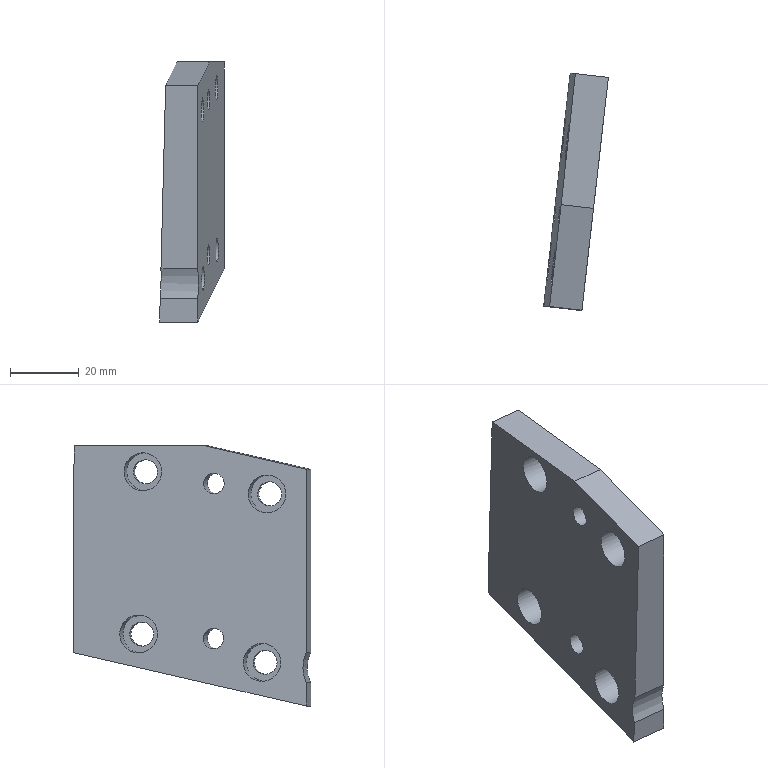Part | NX | features XQ 2 | 1 solid | 23 faces | box 18.804 x 68.828 x 75.49 mm | volume 42663 mm3 | plane 12 | cylinder 11 | commonest cylinder face diameters 7 x4 11 x4 6.001 x2 20 x1
STEP:
#1=CARTESIAN_POINT('',(2657.194,-285.051,-83.004));
#2=VERTEX_POINT('',#1);
#3=CARTESIAN_POINT('',(2656.854,-288.032,-83.004));
#4=DIRECTION('',(-0.9936,0.1132,-0.000000001));
#5=DIRECTION('',(0.1132,0.9936,0.));
#6=AXIS2_PLACEMENT_3D('',#3,#4,#5);
#7=CIRCLE('',#6,3.001);
#8=EDGE_CURVE('',#2,#2,#7,.T.);
#9=ORIENTED_EDGE('',*,*,#8,.T.);
#10=EDGE_LOOP('',(#9));
#11=FACE_BOUND('',#10,.T.);
#12=CARTESIAN_POINT('',(2659.599,-263.939,-34.581));
#13=VERTEX_POINT('',#12);
#14=CARTESIAN_POINT('',(2659.203,-267.417,-34.581));
#15=DIRECTION('',(0.9936,-0.1132,0.000000001));
#16=DIRECTION('',(0.1132,0.9936,0.));
#17=AXIS2_PLACEMENT_3D('',#14,#15,#16);
#18=CIRCLE('',#17,3.5);
#19=EDGE_CURVE('',#13,#13,#18,.T.);
#20=ORIENTED_EDGE('',*,*,#19,.F.);
#21=EDGE_LOOP('',(#20));
#22=FACE_BOUND('',#21,.T.);
#23=CARTESIAN_POINT('',(2655.64,-298.684,-89.911));
#24=VERTEX_POINT('',#23);
#25=CARTESIAN_POINT('',(2655.244,-302.162,-89.911));
#26=DIRECTION('',(0.9936,-0.1132,0.000000001));
#27=DIRECTION('',(0.1132,0.9936,0.));
#28=AXIS2_PLACEMENT_3D('',#25,#26,#27);
#29=CIRCLE('',#28,3.5);
#30=EDGE_CURVE('',#24,#24,#29,.T.);
#31=ORIENTED_EDGE('',*,*,#30,.F.);
#32=EDGE_LOOP('',(#31));
#33=FACE_BOUND('',#32,.T.);
#34=CARTESIAN_POINT('',(2659.724,-262.841,-81.692));
#35=VERTEX_POINT('',#34);
#36=CARTESIAN_POINT('',(2659.328,-266.318,-81.692));
#37=DIRECTION('',(0.9936,-0.1132,0.000000001));
#38=DIRECTION('',(0.1132,0.9936,0.));
#39=AXIS2_PLACEMENT_3D('',#36,#37,#38);
#40=CIRCLE('',#39,3.5);
#41=EDGE_CURVE('',#35,#35,#40,.T.);
#42=ORIENTED_EDGE('',*,*,#41,.F.);
#43=EDGE_LOOP('',(#42));
#44=FACE_BOUND('',#43,.T.);
#45=CARTESIAN_POINT('',(2655.493,-299.982,-41.023));
#46=VERTEX_POINT('',#45);
#47=CARTESIAN_POINT('',(2655.096,-303.459,-41.023));
#48=DIRECTION('',(0.9936,-0.1132,0.000000001));
#49=DIRECTION('',(0.1132,0.9936,0.));
#50=AXIS2_PLACEMENT_3D('',#47,#48,#49);
#51=CIRCLE('',#50,3.5);
#52=EDGE_CURVE('',#46,#46,#51,.T.);
#53=ORIENTED_EDGE('',*,*,#52,.F.);
#54=EDGE_LOOP('',(#53));
#55=FACE_BOUND('',#54,.T.);
#56=CARTESIAN_POINT('',(2653.781,-315.001,-102.59));
#57=VERTEX_POINT('',#56);
#58=CARTESIAN_POINT('',(2661.479,-247.438,-87.098));
#59=VERTEX_POINT('',#58);
#60=CARTESIAN_POINT('',(2503.911,-1630.398,-404.205));
#61=DIRECTION('',(0.1104,0.9687,0.2221));
#62=VECTOR('',#61,1000.);
#63=LINE('',#60,#62);
#64=EDGE_CURVE('',#57,#59,#63,.T.);
#65=ORIENTED_EDGE('',*,*,#64,.T.);
#66=CARTESIAN_POINT('',(2661.479,-247.438,-27.1));
#67=VERTEX_POINT('',#66);
#68=CARTESIAN_POINT('',(2661.479,-247.438,-706.6));
#69=DIRECTION('',(-0.000000001,0.,1.));
#70=VECTOR('',#69,1000.);
#71=LINE('',#68,#70);
#72=EDGE_CURVE('',#59,#67,#71,.T.);
#73=ORIENTED_EDGE('',*,*,#72,.T.);
#74=CARTESIAN_POINT('',(2657.147,-285.463,-27.1));
#75=VERTEX_POINT('',#74);
#76=CARTESIAN_POINT('',(2511.71,-1561.949,-27.1));
#77=DIRECTION('',(-0.1132,-0.9936,0.));
#78=VECTOR('',#77,1000.);
#79=LINE('',#76,#78);
#80=EDGE_CURVE('',#67,#75,#79,.T.);
#81=ORIENTED_EDGE('',*,*,#80,.T.);
#82=CARTESIAN_POINT('',(2653.781,-315.001,-33.873));
#83=VERTEX_POINT('',#82);
#84=CARTESIAN_POINT('',(2502.226,-1645.185,-338.879));
#85=DIRECTION('',(0.1104,0.9687,0.2221));
#86=VECTOR('',#85,1000.);
#87=LINE('',#84,#86);
#88=EDGE_CURVE('',#83,#75,#87,.T.);
#89=ORIENTED_EDGE('',*,*,#88,.F.);
#90=CARTESIAN_POINT('',(2653.781,-315.001,-87.141));
#91=VERTEX_POINT('',#90);
#92=CARTESIAN_POINT('',(2653.781,-315.001,-706.6));
#93=DIRECTION('',(0.000000001,0.,-1.));
#94=VECTOR('',#93,1000.);
#95=LINE('',#92,#94);
#96=EDGE_CURVE('',#83,#91,#95,.T.);
#97=ORIENTED_EDGE('',*,*,#96,.T.);
#98=CARTESIAN_POINT('',(2653.781,-315.001,-95.859));
#99=VERTEX_POINT('',#98);
#100=CARTESIAN_POINT('',(2652.762,-323.943,-91.5));
#101=DIRECTION('',(0.9936,-0.1132,0.000000001));
#102=DIRECTION('',(0.000000001,0.,-1.));
#103=AXIS2_PLACEMENT_3D('',#100,#101,#102);
#104=CIRCLE('',#103,10.);
#105=EDGE_CURVE('',#99,#91,#104,.T.);
#106=ORIENTED_EDGE('',*,*,#105,.F.);
#107=CARTESIAN_POINT('',(2653.781,-315.001,-706.6));
#108=DIRECTION('',(0.000000001,0.,-1.));
#109=VECTOR('',#108,1000.);
#110=LINE('',#107,#109);
#111=EDGE_CURVE('',#99,#57,#110,.T.);
#112=ORIENTED_EDGE('',*,*,#111,.T.);
#113=EDGE_LOOP('',(#65,#73,#81,#89,#97,#106,#112));
#114=FACE_BOUND('',#113,.T.);
#115=CARTESIAN_POINT('',(2657.194,-285.051,-38.004));
#116=VERTEX_POINT('',#115);
#117=CARTESIAN_POINT('',(2656.854,-288.032,-38.004));
#118=DIRECTION('',(-0.9936,0.1132,-0.000000001));
#119=DIRECTION('',(0.1132,0.9936,0.));
#120=AXIS2_PLACEMENT_3D('',#117,#118,#119);
#121=CIRCLE('',#120,3.001);
#122=EDGE_CURVE('',#116,#116,#121,.T.);
#123=ORIENTED_EDGE('',*,*,#122,.T.);
#124=EDGE_LOOP('',(#123));
#125=FACE_BOUND('',#124,.T.);
#126=CARTESIAN_POINT('',(2511.71,-1561.949,-706.6));
#127=DIRECTION('',(0.9936,-0.1132,0.000000001));
#128=DIRECTION('',(0.000000001,0.000000001,-1.));
#129=AXIS2_PLACEMENT_3D('',#126,#127,#128);
#130=PLANE('',#129);
#131=ADVANCED_FACE('',(#11,#22,#33,#44,#55,#114,#125),#130,.T.);
#132=CARTESIAN_POINT('',(2646.085,-286.134,-85.93));
#133=VERTEX_POINT('',#132);
#134=CARTESIAN_POINT('',(2646.087,-286.806,-83.004));
#135=DIRECTION('',(-0.9939,0.1074,0.02552));
#136=DIRECTION('',(-0.0008715,0.2236,-0.9747));
#137=AXIS2_PLACEMENT_3D('',#134,#135,#136);
#138=ELLIPSE('',#137,3.002,3.001);
#139=EDGE_CURVE('',#133,#133,#138,.T.);
#140=ORIENTED_EDGE('',*,*,#139,.F.);
#141=EDGE_LOOP('',(#140));
#142=FACE_BOUND('',#141,.T.);
#143=CARTESIAN_POINT('',(2649.55,-267.547,-29.218));
#144=VERTEX_POINT('',#143);
#145=CARTESIAN_POINT('',(2649.545,-266.316,-34.581));
#146=DIRECTION('',(0.9939,-0.1074,-0.02552));
#147=DIRECTION('',(0.0008715,-0.2236,0.9747));
#148=AXIS2_PLACEMENT_3D('',#145,#146,#147);
#149=ELLIPSE('',#148,5.502,5.5);
#150=EDGE_CURVE('',#144,#144,#149,.T.);
#151=ORIENTED_EDGE('',*,*,#150,.T.);
#152=EDGE_LOOP('',(#151));
#153=FACE_BOUND('',#152,.T.);
#154=CARTESIAN_POINT('',(2644.389,-302.155,-84.548));
#155=VERTEX_POINT('',#154);
#156=CARTESIAN_POINT('',(2644.385,-300.924,-89.911));
#157=DIRECTION('',(0.9939,-0.1074,-0.02552));
#158=DIRECTION('',(0.0008715,-0.2236,0.9747));
#159=AXIS2_PLACEMENT_3D('',#156,#157,#158);
#160=ELLIPSE('',#159,5.502,5.5);
#161=EDGE_CURVE('',#155,#155,#160,.T.);
#162=ORIENTED_EDGE('',*,*,#161,.T.);
#163=EDGE_LOOP('',(#162));
#164=FACE_BOUND('',#163,.T.);
#165=CARTESIAN_POINT('',(2648.473,-266.311,-76.33));
#166=VERTEX_POINT('',#165);
#167=CARTESIAN_POINT('',(2648.468,-265.081,-81.692));
#168=DIRECTION('',(0.9939,-0.1074,-0.02552));
#169=DIRECTION('',(0.0008715,-0.2236,0.9747));
#170=AXIS2_PLACEMENT_3D('',#167,#168,#169);
#171=ELLIPSE('',#170,5.502,5.5);
#172=EDGE_CURVE('',#166,#166,#171,.T.);
#173=ORIENTED_EDGE('',*,*,#172,.T.);
#174=EDGE_LOOP('',(#173));
#175=FACE_BOUND('',#174,.T.);
#176=CARTESIAN_POINT('',(2645.489,-303.594,-35.66));
#177=VERTEX_POINT('',#176);
#178=CARTESIAN_POINT('',(2645.484,-302.364,-41.023));
#179=DIRECTION('',(0.9939,-0.1074,-0.02552));
#180=DIRECTION('',(0.0008715,-0.2236,0.9747));
#181=AXIS2_PLACEMENT_3D('',#178,#179,#180);
#182=ELLIPSE('',#181,5.502,5.5);
#183=EDGE_CURVE('',#177,#177,#182,.T.);
#184=ORIENTED_EDGE('',*,*,#183,.T.);
#185=EDGE_LOOP('',(#184));
#186=FACE_BOUND('',#185,.T.);
#187=CARTESIAN_POINT('',(2650.373,-246.173,-87.098));
#188=VERTEX_POINT('',#187);
#189=CARTESIAN_POINT('',(2651.895,-246.346,-27.1));
#190=VERTEX_POINT('',#189);
#191=CARTESIAN_POINT('',(2634.665,-244.383,-706.285));
#192=DIRECTION('',(0.02536,-0.002889,0.9997));
#193=VECTOR('',#192,1000.);
#194=LINE('',#191,#193);
#195=EDGE_CURVE('',#188,#190,#194,.T.);
#196=ORIENTED_EDGE('',*,*,#195,.F.);
#197=CARTESIAN_POINT('',(2642.675,-313.736,-102.59));
#198=VERTEX_POINT('',#197);
#199=CARTESIAN_POINT('',(2492.804,-1629.133,-404.205));
#200=DIRECTION('',(0.1104,0.9687,0.2221));
#201=VECTOR('',#200,1000.);
#202=LINE('',#199,#201);
#203=EDGE_CURVE('',#198,#188,#202,.T.);
#204=ORIENTED_EDGE('',*,*,#203,.F.);
#205=CARTESIAN_POINT('',(2642.845,-313.755,-95.859));
#206=VERTEX_POINT('',#205);
#207=CARTESIAN_POINT('',(2643.265,-313.803,-79.312));
#208=DIRECTION('',(0.02536,-0.002889,0.9997));
#209=VECTOR('',#208,1000.);
#210=LINE('',#207,#209);
#211=EDGE_CURVE('',#198,#206,#210,.T.);
#212=ORIENTED_EDGE('',*,*,#211,.T.);
#213=CARTESIAN_POINT('',(2643.067,-313.78,-87.141));
#214=VERTEX_POINT('',#213);
#215=CARTESIAN_POINT('',(2641.989,-322.716,-91.5));
#216=DIRECTION('',(0.9939,-0.1074,-0.02552));
#217=DIRECTION('',(-0.0008715,0.2236,-0.9747));
#218=AXIS2_PLACEMENT_3D('',#215,#216,#217);
#219=ELLIPSE('',#218,10.003,10.);
#220=EDGE_CURVE('',#206,#214,#219,.T.);
#221=ORIENTED_EDGE('',*,*,#220,.T.);
#222=CARTESIAN_POINT('',(2644.418,-313.934,-33.873));
#223=VERTEX_POINT('',#222);
#224=CARTESIAN_POINT('',(2643.265,-313.803,-79.312));
#225=DIRECTION('',(0.02536,-0.002889,0.9997));
#226=VECTOR('',#225,1000.);
#227=LINE('',#224,#226);
#228=EDGE_CURVE('',#214,#223,#227,.T.);
#229=ORIENTED_EDGE('',*,*,#228,.T.);
#230=CARTESIAN_POINT('',(2647.783,-284.396,-27.1));
#231=VERTEX_POINT('',#230);
#232=CARTESIAN_POINT('',(2492.863,-1644.118,-338.879));
#233=DIRECTION('',(0.1104,0.9687,0.2221));
#234=VECTOR('',#233,1000.);
#235=LINE('',#232,#234);
#236=EDGE_CURVE('',#223,#231,#235,.T.);
#237=ORIENTED_EDGE('',*,*,#236,.T.);
#238=CARTESIAN_POINT('',(2509.779,-1561.654,-27.1));
#239=DIRECTION('',(-0.1074,-0.9942,0.));
#240=VECTOR('',#239,1000.);
#241=LINE('',#238,#240);
#242=EDGE_CURVE('',#190,#231,#241,.T.);
#243=ORIENTED_EDGE('',*,*,#242,.F.);
#244=EDGE_LOOP('',(#196,#204,#212,#221,#229,#237,#243));
#245=FACE_BOUND('',#244,.T.);
#246=CARTESIAN_POINT('',(2647.226,-286.265,-40.93));
#247=VERTEX_POINT('',#246);
#248=CARTESIAN_POINT('',(2647.229,-286.936,-38.004));
#249=DIRECTION('',(-0.9939,0.1074,0.02552));
#250=DIRECTION('',(-0.0008715,0.2236,-0.9747));
#251=AXIS2_PLACEMENT_3D('',#248,#249,#250);
#252=ELLIPSE('',#251,3.002,3.001);
#253=EDGE_CURVE('',#247,#247,#252,.T.);
#254=ORIENTED_EDGE('',*,*,#253,.F.);
#255=EDGE_LOOP('',(#254));
#256=FACE_BOUND('',#255,.T.);
#257=CARTESIAN_POINT('',(2492.534,-1559.791,-706.481));
#258=DIRECTION('',(0.9939,-0.1074,-0.02552));
#259=DIRECTION('',(-0.02537,0.002816,-0.9997));
#260=AXIS2_PLACEMENT_3D('',#257,#258,#259);
#261=PLANE('',#260);
#262=ADVANCED_FACE('',(#142,#153,#164,#175,#186,#245,#256),#261,.F.);
#263=CARTESIAN_POINT('',(2652.071,-303.513,-44.5));
#264=VERTEX_POINT('',#263);
#265=CARTESIAN_POINT('',(2652.116,-303.119,-41.023));
#266=DIRECTION('',(0.9936,-0.1132,0.));
#267=DIRECTION('',(-0.01281,-0.1125,-0.9936));
#268=AXIS2_PLACEMENT_3D('',#265,#266,#267);
#269=CIRCLE('',#268,3.5);
#270=EDGE_CURVE('',#264,#264,#269,.T.);
#271=ORIENTED_EDGE('',*,*,#270,.T.);
#272=EDGE_LOOP('',(#271));
#273=FACE_BOUND('',#272,.T.);
#274=CARTESIAN_POINT('',(2652.186,-302.501,-35.558));
#275=VERTEX_POINT('',#274);
#276=CARTESIAN_POINT('',(2652.116,-303.119,-41.023));
#277=DIRECTION('',(0.9936,-0.1132,0.));
#278=DIRECTION('',(0.01281,0.1125,0.9936));
#279=AXIS2_PLACEMENT_3D('',#276,#277,#278);
#280=CIRCLE('',#279,5.5);
#281=EDGE_CURVE('',#275,#275,#280,.T.);
#282=ORIENTED_EDGE('',*,*,#281,.F.);
#283=EDGE_LOOP('',(#282));
#284=FACE_BOUND('',#283,.T.);
#285=CARTESIAN_POINT('',(2654.875,-278.901,-37.469));
#286=DIRECTION('',(0.9936,-0.1132,0.));
#287=DIRECTION('',(0.01281,0.1125,0.9936));
#288=AXIS2_PLACEMENT_3D('',#285,#286,#287);
#289=PLANE('',#288);
#290=ADVANCED_FACE('',(#273,#284),#289,.F.);
#291=CARTESIAN_POINT('',(2656.302,-266.372,-85.17));
#292=VERTEX_POINT('',#291);
#293=CARTESIAN_POINT('',(2656.347,-265.978,-81.692));
#294=DIRECTION('',(0.9936,-0.1132,0.));
#295=DIRECTION('',(-0.01281,-0.1125,-0.9936));
#296=AXIS2_PLACEMENT_3D('',#293,#294,#295);
#297=CIRCLE('',#296,3.5);
#298=EDGE_CURVE('',#292,#292,#297,.T.);
#299=ORIENTED_EDGE('',*,*,#298,.T.);
#300=EDGE_LOOP('',(#299));
#301=FACE_BOUND('',#300,.T.);
#302=CARTESIAN_POINT('',(2656.418,-265.36,-76.228));
#303=VERTEX_POINT('',#302);
#304=CARTESIAN_POINT('',(2656.347,-265.978,-81.692));
#305=DIRECTION('',(0.9936,-0.1132,0.));
#306=DIRECTION('',(0.01281,0.1125,0.9936));
#307=AXIS2_PLACEMENT_3D('',#304,#305,#306);
#308=CIRCLE('',#307,5.5);
#309=EDGE_CURVE('',#303,#303,#308,.T.);
#310=ORIENTED_EDGE('',*,*,#309,.F.);
#311=EDGE_LOOP('',(#310));
#312=FACE_BOUND('',#311,.T.);
#313=CARTESIAN_POINT('',(2654.25,-284.385,-85.913));
#314=DIRECTION('',(0.9936,-0.1132,0.));
#315=DIRECTION('',(0.01281,0.1125,0.9936));
#316=AXIS2_PLACEMENT_3D('',#313,#314,#315);
#317=PLANE('',#316);
#318=ADVANCED_FACE('',(#301,#312),#317,.F.);
#319=CARTESIAN_POINT('',(2652.219,-302.216,-93.389));
#320=VERTEX_POINT('',#319);
#321=CARTESIAN_POINT('',(2652.263,-301.822,-89.911));
#322=DIRECTION('',(0.9936,-0.1132,0.));
#323=DIRECTION('',(-0.01281,-0.1125,-0.9936));
#324=AXIS2_PLACEMENT_3D('',#321,#322,#323);
#325=CIRCLE('',#324,3.5);
#326=EDGE_CURVE('',#320,#320,#325,.T.);
#327=ORIENTED_EDGE('',*,*,#326,.T.);
#328=EDGE_LOOP('',(#327));
#329=FACE_BOUND('',#328,.T.);
#330=CARTESIAN_POINT('',(2652.334,-301.204,-84.446));
#331=VERTEX_POINT('',#330);
#332=CARTESIAN_POINT('',(2652.263,-301.822,-89.911));
#333=DIRECTION('',(0.9936,-0.1132,0.));
#334=DIRECTION('',(0.01281,0.1125,0.9936));
#335=AXIS2_PLACEMENT_3D('',#332,#333,#334);
#336=CIRCLE('',#335,5.5);
#337=EDGE_CURVE('',#331,#331,#336,.T.);
#338=ORIENTED_EDGE('',*,*,#337,.F.);
#339=EDGE_LOOP('',(#338));
#340=FACE_BOUND('',#339,.T.);
#341=CARTESIAN_POINT('',(2652.263,-301.822,-89.911));
#342=DIRECTION('',(0.9936,-0.1132,0.));
#343=DIRECTION('',(0.01281,0.1125,0.9936));
#344=AXIS2_PLACEMENT_3D('',#341,#342,#343);
#345=PLANE('',#344);
#346=ADVANCED_FACE('',(#329,#340),#345,.F.);
#347=CARTESIAN_POINT('',(2651.297,-314.718,-102.59));
#348=DIRECTION('',(-0.9936,0.1132,-0.000000001));
#349=VECTOR('',#348,1000.);
#350=LINE('',#347,#349);
#351=EDGE_CURVE('',#57,#198,#350,.T.);
#352=ORIENTED_EDGE('',*,*,#351,.F.);
#353=ORIENTED_EDGE('',*,*,#111,.F.);
#354=CARTESIAN_POINT('',(3066.114,-361.98,-95.859));
#355=DIRECTION('',(-0.9936,0.1132,-0.000000001));
#356=VECTOR('',#355,1000.);
#357=LINE('',#354,#356);
#358=EDGE_CURVE('',#99,#206,#357,.T.);
#359=ORIENTED_EDGE('',*,*,#358,.T.);
#360=ORIENTED_EDGE('',*,*,#211,.F.);
#361=EDGE_LOOP('',(#352,#353,#359,#360));
#362=FACE_BOUND('',#361,.T.);
#363=CARTESIAN_POINT('',(2648.813,-314.435,-79.455));
#364=DIRECTION('',(-0.1132,-0.9936,0.));
#365=DIRECTION('',(-0.9936,0.1132,0.));
#366=AXIS2_PLACEMENT_3D('',#363,#364,#365);
#367=PLANE('',#366);
#368=ADVANCED_FACE('',(#362),#367,.T.);
#369=ORIENTED_EDGE('',*,*,#105,.T.);
#370=CARTESIAN_POINT('',(3066.114,-361.98,-87.141));
#371=DIRECTION('',(0.9936,-0.1132,0.000000001));
#372=VECTOR('',#371,1000.);
#373=LINE('',#370,#372);
#374=EDGE_CURVE('',#214,#91,#373,.T.);
#375=ORIENTED_EDGE('',*,*,#374,.F.);
#376=ORIENTED_EDGE('',*,*,#220,.F.);
#377=ORIENTED_EDGE('',*,*,#358,.F.);
#378=EDGE_LOOP('',(#369,#375,#376,#377));
#379=FACE_BOUND('',#378,.T.);
#380=CARTESIAN_POINT('',(3065.095,-370.923,-91.5));
#381=DIRECTION('',(-0.9936,0.1132,-0.000000001));
#382=DIRECTION('',(0.000000001,0.,-1.));
#383=AXIS2_PLACEMENT_3D('',#380,#381,#382);
#384=CYLINDRICAL_SURFACE('',#383,10.);
#385=ADVANCED_FACE('',(#379),#384,.F.);
#386=ORIENTED_EDGE('',*,*,#96,.F.);
#387=CARTESIAN_POINT('',(2658.749,-315.567,-33.873));
#388=DIRECTION('',(-0.9936,0.1132,-0.000000001));
#389=VECTOR('',#388,1000.);
#390=LINE('',#387,#389);
#391=EDGE_CURVE('',#83,#223,#390,.T.);
#392=ORIENTED_EDGE('',*,*,#391,.T.);
#393=ORIENTED_EDGE('',*,*,#228,.F.);
#394=ORIENTED_EDGE('',*,*,#374,.T.);
#395=EDGE_LOOP('',(#386,#392,#393,#394));
#396=FACE_BOUND('',#395,.T.);
#397=CARTESIAN_POINT('',(2648.813,-314.435,-79.455));
#398=DIRECTION('',(-0.1132,-0.9936,0.));
#399=DIRECTION('',(-0.9936,0.1132,0.));
#400=AXIS2_PLACEMENT_3D('',#397,#398,#399);
#401=PLANE('',#400);
#402=ADVANCED_FACE('',(#396),#401,.T.);
#403=ORIENTED_EDGE('',*,*,#391,.F.);
#404=ORIENTED_EDGE('',*,*,#88,.T.);
#405=CARTESIAN_POINT('',(2662.115,-286.029,-27.1));
#406=DIRECTION('',(0.9936,-0.1132,0.));
#407=VECTOR('',#406,1000.);
#408=LINE('',#405,#407);
#409=EDGE_CURVE('',#231,#75,#408,.T.);
#410=ORIENTED_EDGE('',*,*,#409,.F.);
#411=ORIENTED_EDGE('',*,*,#236,.F.);
#412=EDGE_LOOP('',(#403,#404,#410,#411));
#413=FACE_BOUND('',#412,.T.);
#414=CARTESIAN_POINT('',(2659.211,-311.513,-32.943));
#415=DIRECTION('',(-0.02515,-0.2207,0.975));
#416=DIRECTION('',(0.,0.9753,0.2208));
#417=AXIS2_PLACEMENT_3D('',#414,#415,#416);
#418=PLANE('',#417);
#419=ADVANCED_FACE('',(#413),#418,.T.);
#420=ORIENTED_EDGE('',*,*,#80,.F.);
#421=CARTESIAN_POINT('',(2651.543,-246.306,-27.1));
#422=DIRECTION('',(-0.9936,0.1132,0.));
#423=VECTOR('',#422,1000.);
#424=LINE('',#421,#423);
#425=EDGE_CURVE('',#67,#190,#424,.T.);
#426=ORIENTED_EDGE('',*,*,#425,.T.);
#427=ORIENTED_EDGE('',*,*,#242,.T.);
#428=ORIENTED_EDGE('',*,*,#409,.T.);
#429=EDGE_LOOP('',(#420,#426,#427,#428));
#430=FACE_BOUND('',#429,.T.);
#431=CARTESIAN_POINT('',(2656.658,-201.414,-27.1));
#432=DIRECTION('',(0.,0.,1.));
#433=DIRECTION('',(-1.,0.,0.));
#434=AXIS2_PLACEMENT_3D('',#431,#432,#433);
#435=PLANE('',#434);
#436=ADVANCED_FACE('',(#430),#435,.T.);
#437=CARTESIAN_POINT('',(2658.995,-247.155,-87.098));
#438=DIRECTION('',(-0.9936,0.1132,-0.000000001));
#439=VECTOR('',#438,1000.);
#440=LINE('',#437,#439);
#441=EDGE_CURVE('',#59,#188,#440,.T.);
#442=ORIENTED_EDGE('',*,*,#441,.T.);
#443=ORIENTED_EDGE('',*,*,#195,.T.);
#444=ORIENTED_EDGE('',*,*,#425,.F.);
#445=ORIENTED_EDGE('',*,*,#72,.F.);
#446=EDGE_LOOP('',(#442,#443,#444,#445));
#447=FACE_BOUND('',#446,.T.);
#448=CARTESIAN_POINT('',(2656.511,-246.872,-49.581));
#449=DIRECTION('',(0.1132,0.9936,0.));
#450=DIRECTION('',(0.9936,-0.1132,0.));
#451=AXIS2_PLACEMENT_3D('',#448,#449,#450);
#452=PLANE('',#451);
#453=ADVANCED_FACE('',(#447),#452,.T.);
#454=ORIENTED_EDGE('',*,*,#203,.T.);
#455=ORIENTED_EDGE('',*,*,#441,.F.);
#456=ORIENTED_EDGE('',*,*,#64,.F.);
#457=ORIENTED_EDGE('',*,*,#351,.T.);
#458=EDGE_LOOP('',(#454,#455,#456,#457));
#459=FACE_BOUND('',#458,.T.);
#460=CARTESIAN_POINT('',(2652.739,-302.066,-99.689));
#461=DIRECTION('',(0.02515,0.2207,-0.975));
#462=DIRECTION('',(0.,-0.9753,-0.2208));
#463=AXIS2_PLACEMENT_3D('',#460,#461,#462);
#464=PLANE('',#463);
#465=ADVANCED_FACE('',(#459),#464,.T.);
#466=ORIENTED_EDGE('',*,*,#52,.T.);
#467=EDGE_LOOP('',(#466));
#468=FACE_BOUND('',#467,.T.);
#469=ORIENTED_EDGE('',*,*,#270,.F.);
#470=EDGE_LOOP('',(#469));
#471=FACE_BOUND('',#470,.T.);
#472=CARTESIAN_POINT('',(2643.173,-302.101,-41.023));
#473=DIRECTION('',(0.9936,-0.1132,0.));
#474=DIRECTION('',(-0.01281,-0.1125,-0.9936));
#475=AXIS2_PLACEMENT_3D('',#472,#473,#474);
#476=CYLINDRICAL_SURFACE('',#475,3.5);
#477=ADVANCED_FACE('',(#468,#471),#476,.F.);
#478=ORIENTED_EDGE('',*,*,#41,.T.);
#479=EDGE_LOOP('',(#478));
#480=FACE_BOUND('',#479,.T.);
#481=ORIENTED_EDGE('',*,*,#298,.F.);
#482=EDGE_LOOP('',(#481));
#483=FACE_BOUND('',#482,.T.);
#484=CARTESIAN_POINT('',(2647.405,-264.96,-81.692));
#485=DIRECTION('',(0.9936,-0.1132,0.));
#486=DIRECTION('',(-0.01281,-0.1125,-0.9936));
#487=AXIS2_PLACEMENT_3D('',#484,#485,#486);
#488=CYLINDRICAL_SURFACE('',#487,3.5);
#489=ADVANCED_FACE('',(#480,#483),#488,.F.);
#490=ORIENTED_EDGE('',*,*,#30,.T.);
#491=EDGE_LOOP('',(#490));
#492=FACE_BOUND('',#491,.T.);
#493=ORIENTED_EDGE('',*,*,#326,.F.);
#494=EDGE_LOOP('',(#493));
#495=FACE_BOUND('',#494,.T.);
#496=CARTESIAN_POINT('',(2643.321,-300.803,-89.911));
#497=DIRECTION('',(0.9936,-0.1132,0.));
#498=DIRECTION('',(-0.01281,-0.1125,-0.9936));
#499=AXIS2_PLACEMENT_3D('',#496,#497,#498);
#500=CYLINDRICAL_SURFACE('',#499,3.5);
#501=ADVANCED_FACE('',(#492,#495),#500,.F.);
#502=ORIENTED_EDGE('',*,*,#281,.T.);
#503=EDGE_LOOP('',(#502));
#504=FACE_BOUND('',#503,.T.);
#505=ORIENTED_EDGE('',*,*,#183,.F.);
#506=EDGE_LOOP('',(#505));
#507=FACE_BOUND('',#506,.T.);
#508=CARTESIAN_POINT('',(2645.161,-302.327,-41.023));
#509=DIRECTION('',(0.9936,-0.1132,0.));
#510=DIRECTION('',(-0.01281,-0.1125,-0.9936));
#511=AXIS2_PLACEMENT_3D('',#508,#509,#510);
#512=CYLINDRICAL_SURFACE('',#511,5.5);
#513=ADVANCED_FACE('',(#504,#507),#512,.F.);
#514=ORIENTED_EDGE('',*,*,#309,.T.);
#515=EDGE_LOOP('',(#514));
#516=FACE_BOUND('',#515,.T.);
#517=ORIENTED_EDGE('',*,*,#172,.F.);
#518=EDGE_LOOP('',(#517));
#519=FACE_BOUND('',#518,.T.);
#520=CARTESIAN_POINT('',(2649.392,-265.186,-81.692));
#521=DIRECTION('',(0.9936,-0.1132,0.));
#522=DIRECTION('',(-0.01281,-0.1125,-0.9936));
#523=AXIS2_PLACEMENT_3D('',#520,#521,#522);
#524=CYLINDRICAL_SURFACE('',#523,5.5);
#525=ADVANCED_FACE('',(#516,#519),#524,.F.);
#526=ORIENTED_EDGE('',*,*,#337,.T.);
#527=EDGE_LOOP('',(#526));
#528=FACE_BOUND('',#527,.T.);
#529=ORIENTED_EDGE('',*,*,#161,.F.);
#530=EDGE_LOOP('',(#529));
#531=FACE_BOUND('',#530,.T.);
#532=CARTESIAN_POINT('',(2645.308,-301.03,-89.911));
#533=DIRECTION('',(0.9936,-0.1132,0.));
#534=DIRECTION('',(-0.01281,-0.1125,-0.9936));
#535=AXIS2_PLACEMENT_3D('',#532,#533,#534);
#536=CYLINDRICAL_SURFACE('',#535,5.5);
#537=ADVANCED_FACE('',(#528,#531),#536,.F.);
#538=CARTESIAN_POINT('',(2656.177,-267.471,-38.058));
#539=VERTEX_POINT('',#538);
#540=CARTESIAN_POINT('',(2656.222,-267.077,-34.581));
#541=DIRECTION('',(0.9936,-0.1132,0.));
#542=DIRECTION('',(-0.01281,-0.1125,-0.9936));
#543=AXIS2_PLACEMENT_3D('',#540,#541,#542);
#544=CIRCLE('',#543,3.5);
#545=EDGE_CURVE('',#539,#539,#544,.T.);
#546=ORIENTED_EDGE('',*,*,#545,.T.);
#547=EDGE_LOOP('',(#546));
#548=FACE_BOUND('',#547,.T.);
#549=CARTESIAN_POINT('',(2656.293,-266.459,-29.116));
#550=VERTEX_POINT('',#549);
#551=CARTESIAN_POINT('',(2656.222,-267.077,-34.581));
#552=DIRECTION('',(0.9936,-0.1132,0.));
#553=DIRECTION('',(0.01281,0.1125,0.9936));
#554=AXIS2_PLACEMENT_3D('',#551,#552,#553);
#555=CIRCLE('',#554,5.5);
#556=EDGE_CURVE('',#550,#550,#555,.T.);
#557=ORIENTED_EDGE('',*,*,#556,.F.);
#558=EDGE_LOOP('',(#557));
#559=FACE_BOUND('',#558,.T.);
#560=CARTESIAN_POINT('',(2658.076,-250.807,-31.028));
#561=DIRECTION('',(0.9936,-0.1132,0.));
#562=DIRECTION('',(0.01281,0.1125,0.9936));
#563=AXIS2_PLACEMENT_3D('',#560,#561,#562);
#564=PLANE('',#563);
#565=ADVANCED_FACE('',(#548,#559),#564,.F.);
#566=ORIENTED_EDGE('',*,*,#19,.T.);
#567=EDGE_LOOP('',(#566));
#568=FACE_BOUND('',#567,.T.);
#569=ORIENTED_EDGE('',*,*,#545,.F.);
#570=EDGE_LOOP('',(#569));
#571=FACE_BOUND('',#570,.T.);
#572=CARTESIAN_POINT('',(2647.28,-266.058,-34.581));
#573=DIRECTION('',(0.9936,-0.1132,0.));
#574=DIRECTION('',(-0.01281,-0.1125,-0.9936));
#575=AXIS2_PLACEMENT_3D('',#572,#573,#574);
#576=CYLINDRICAL_SURFACE('',#575,3.5);
#577=ADVANCED_FACE('',(#568,#571),#576,.F.);
#578=ORIENTED_EDGE('',*,*,#556,.T.);
#579=EDGE_LOOP('',(#578));
#580=FACE_BOUND('',#579,.T.);
#581=ORIENTED_EDGE('',*,*,#150,.F.);
#582=EDGE_LOOP('',(#581));
#583=FACE_BOUND('',#582,.T.);
#584=CARTESIAN_POINT('',(2649.267,-266.285,-34.581));
#585=DIRECTION('',(0.9936,-0.1132,0.));
#586=DIRECTION('',(-0.01281,-0.1125,-0.9936));
#587=AXIS2_PLACEMENT_3D('',#584,#585,#586);
#588=CYLINDRICAL_SURFACE('',#587,5.5);
#589=ADVANCED_FACE('',(#580,#583),#588,.F.);
#590=ORIENTED_EDGE('',*,*,#8,.F.);
#591=EDGE_LOOP('',(#590));
#592=FACE_BOUND('',#591,.T.);
#593=ORIENTED_EDGE('',*,*,#139,.T.);
#594=EDGE_LOOP('',(#593));
#595=FACE_BOUND('',#594,.T.);
#596=CARTESIAN_POINT('',(2662.815,-288.711,-83.004));
#597=DIRECTION('',(-0.9936,0.1132,-0.000000001));
#598=DIRECTION('',(0.1132,0.9936,0.));
#599=AXIS2_PLACEMENT_3D('',#596,#597,#598);
#600=CYLINDRICAL_SURFACE('',#599,3.001);
#601=ADVANCED_FACE('',(#592,#595),#600,.F.);
#602=ORIENTED_EDGE('',*,*,#122,.F.);
#603=EDGE_LOOP('',(#602));
#604=FACE_BOUND('',#603,.T.);
#605=ORIENTED_EDGE('',*,*,#253,.T.);
#606=EDGE_LOOP('',(#605));
#607=FACE_BOUND('',#606,.T.);
#608=CARTESIAN_POINT('',(2662.815,-288.711,-38.004));
#609=DIRECTION('',(-0.9936,0.1132,-0.000000001));
#610=DIRECTION('',(0.1132,0.9936,0.));
#611=AXIS2_PLACEMENT_3D('',#608,#609,#610);
#612=CYLINDRICAL_SURFACE('',#611,3.001);
#613=ADVANCED_FACE('',(#604,#607),#612,.F.);
#614=CLOSED_SHELL('',(#131,#262,#290,#318,#346,#368,#385,#402,#419,#436,#453,#465,#477,#489,#501,#513,#525,#537,#565,#577,#589,#601,#613));
#615=MANIFOLD_SOLID_BREP('',#614);
#616=(LENGTH_UNIT()NAMED_UNIT(*)SI_UNIT(.MILLI.,.METRE.));
#617=UNCERTAINTY_MEASURE_WITH_UNIT(LENGTH_MEASURE(0.00001),#616,'','');
#618=(NAMED_UNIT(*)PLANE_ANGLE_UNIT()SI_UNIT($,.RADIAN.));
#619=(NAMED_UNIT(*)SI_UNIT($,.STERADIAN.)SOLID_ANGLE_UNIT());
#620=(GEOMETRIC_REPRESENTATION_CONTEXT(3)GLOBAL_UNCERTAINTY_ASSIGNED_CONTEXT((#617))GLOBAL_UNIT_ASSIGNED_CONTEXT((#616,#618,#619))REPRESENTATION_CONTEXT('',''));
#621=ADVANCED_BREP_SHAPE_REPRESENTATION('',(#615),#620);